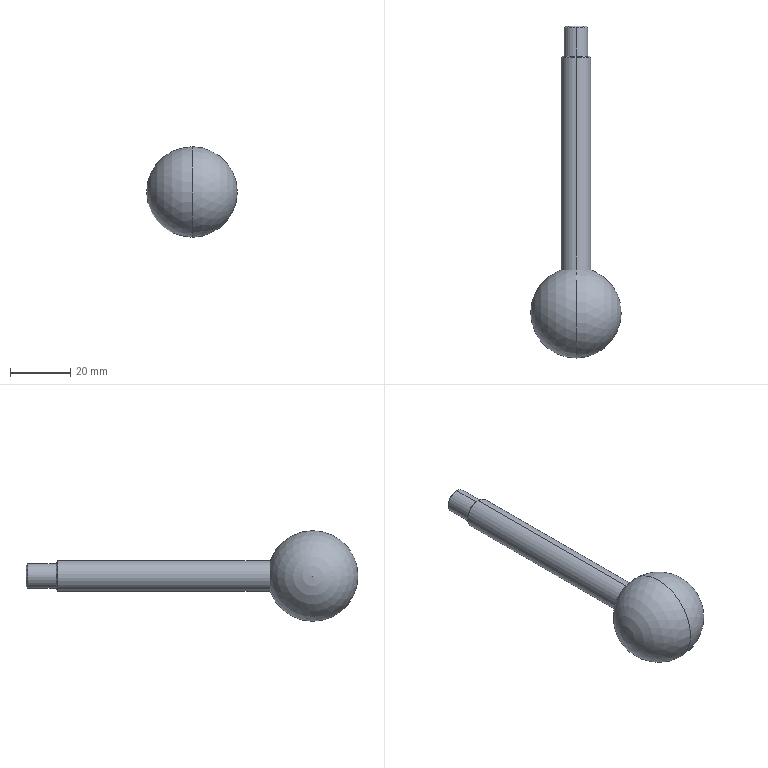Part | STEP file | M8 handle_SUS304 | 1 solid | 12 faces | box 30 x 110 x 30 mm | volume 20164 mm3 | cylinder 4 | cone 4 | sphere 2 | plane 2 | commonest cylinder face diameters 8 x2 10 x2
STEP:
#1=CARTESIAN_POINT('',(0.,0.,0.));
#2=DIRECTION('',(0.,0.,1.));
#3=DIRECTION('',(1.,0.,0.));
#4=AXIS2_PLACEMENT_3D('',#1,#2,#3);
#5=CARTESIAN_POINT('',(0.,-15.,0.));
#6=VERTEX_POINT('',#5);
#7=CARTESIAN_POINT('',(0.,0.,15.));
#8=VERTEX_POINT('',#7);
#9=CARTESIAN_POINT('',(0.,0.,0.));
#10=DIRECTION('',(-1.,0.,0.));
#11=DIRECTION('',(0.,-1.,0.));
#12=AXIS2_PLACEMENT_3D('',#9,#10,#11);
#13=CIRCLE('',#12,15.);
#14=CARTESIAN_POINT('',(0.,0.,0.));
#15=DIRECTION('',(1.,0.,0.));
#16=DIRECTION('',(0.,-1.,0.));
#17=AXIS2_PLACEMENT_3D('',#14,#15,#16);
#18=SPHERICAL_SURFACE('',#17,15.);
#19=CARTESIAN_POINT('',(6.283,0.));
#20=CARTESIAN_POINT('',(6.236,0.));
#21=CARTESIAN_POINT('',(6.14,0.));
#22=CARTESIAN_POINT('',(5.998,0.));
#23=CARTESIAN_POINT('',(5.855,0.));
#24=CARTESIAN_POINT('',(5.712,0.));
#25=CARTESIAN_POINT('',(5.569,0.));
#26=CARTESIAN_POINT('',(5.426,0.));
#27=CARTESIAN_POINT('',(5.284,0.));
#28=CARTESIAN_POINT('',(5.141,0.));
#29=CARTESIAN_POINT('',(4.998,0.));
#30=CARTESIAN_POINT('',(4.855,0.));
#31=CARTESIAN_POINT('',(4.76,0.));
#32=CARTESIAN_POINT('',(4.712,0.));
#33=B_SPLINE_CURVE_WITH_KNOTS('',3,(#19,#20,#21,#22,#23,#24,#25,#26,#27,#28,#29,#30,#31,#32),.UNSPECIFIED.,.F.,.F.,(4,1,1,1,1,1,1,1,1,1,1,4),(0.,0.1428,0.2856,0.4284,0.5712,0.714,0.8568,0.9996,1.142,1.285,1.428,1.571),.QUASI_UNIFORM_KNOTS.);
#34=(GEOMETRIC_REPRESENTATION_CONTEXT(2)PARAMETRIC_REPRESENTATION_CONTEXT()REPRESENTATION_CONTEXT('',''));
#35=DEFINITIONAL_REPRESENTATION('',(#33),#34);
#36=PCURVE('',#18,#35);
#37=CARTESIAN_POINT('',(0.,0.,0.));
#38=DIRECTION('',(1.,0.,0.));
#39=DIRECTION('',(0.,-1.,0.));
#40=AXIS2_PLACEMENT_3D('',#37,#38,#39);
#41=SPHERICAL_SURFACE('',#40,15.);
#42=CARTESIAN_POINT('',(6.283,0.));
#43=CARTESIAN_POINT('',(6.259,0.));
#44=CARTESIAN_POINT('',(6.212,0.));
#45=CARTESIAN_POINT('',(6.14,0.));
#46=CARTESIAN_POINT('',(6.069,0.));
#47=CARTESIAN_POINT('',(5.998,0.));
#48=CARTESIAN_POINT('',(5.926,0.));
#49=CARTESIAN_POINT('',(5.855,0.));
#50=CARTESIAN_POINT('',(5.783,0.));
#51=CARTESIAN_POINT('',(5.712,0.));
#52=CARTESIAN_POINT('',(5.641,0.));
#53=CARTESIAN_POINT('',(5.569,0.));
#54=CARTESIAN_POINT('',(5.498,0.));
#55=CARTESIAN_POINT('',(5.426,0.));
#56=CARTESIAN_POINT('',(5.355,0.));
#57=CARTESIAN_POINT('',(5.284,0.));
#58=CARTESIAN_POINT('',(5.212,0.));
#59=CARTESIAN_POINT('',(5.141,0.));
#60=CARTESIAN_POINT('',(5.069,0.));
#61=CARTESIAN_POINT('',(4.998,0.));
#62=CARTESIAN_POINT('',(4.927,0.));
#63=CARTESIAN_POINT('',(4.855,0.));
#64=CARTESIAN_POINT('',(4.784,0.));
#65=CARTESIAN_POINT('',(4.736,0.));
#66=CARTESIAN_POINT('',(4.712,0.));
#67=B_SPLINE_CURVE_WITH_KNOTS('',3,(#42,#43,#44,#45,#46,#47,#48,#49,#50,#51,#52,#53,#54,#55,#56,#57,#58,#59,#60,#61,#62,#63,#64,#65,#66),.UNSPECIFIED.,.F.,.F.,(4,1,1,1,1,1,1,1,1,1,1,1,1,1,1,1,1,1,1,1,1,1,4),(0.,0.0714,0.1428,0.2142,0.2856,0.357,0.4284,0.4998,0.5712,0.6426,0.714,0.7854,0.8568,0.9282,0.9996,1.071,1.142,1.214,1.285,1.357,1.428,1.499,1.571),.QUASI_UNIFORM_KNOTS.);
#68=(GEOMETRIC_REPRESENTATION_CONTEXT(2)PARAMETRIC_REPRESENTATION_CONTEXT()REPRESENTATION_CONTEXT('',''));
#69=DEFINITIONAL_REPRESENTATION('',(#67),#68);
#70=PCURVE('',#41,#69);
#71=SURFACE_CURVE('',#13,(#36,#70),.PCURVE_S1.);
#72=EDGE_CURVE('',#6,#8,#71,.T.);
#73=ORIENTED_EDGE('',*,*,#72,.F.);
#74=CARTESIAN_POINT('',(15.,0.,0.));
#75=VERTEX_POINT('',#74);
#76=CARTESIAN_POINT('',(0.,-15.,0.));
#77=CARTESIAN_POINT('',(3.366,-15.,0.));
#78=CARTESIAN_POINT('',(6.732,-14.119,0.));
#79=CARTESIAN_POINT('',(9.821,-12.356,0.));
#80=CARTESIAN_POINT('',(12.356,-9.821,0.));
#81=CARTESIAN_POINT('',(14.119,-6.732,0.));
#82=CARTESIAN_POINT('',(15.,-3.366,0.));
#83=CARTESIAN_POINT('',(15.,0.,0.));
#84=B_SPLINE_CURVE_WITH_KNOTS('',7,(#76,#77,#78,#79,#80,#81,#82,#83),.UNSPECIFIED.,.F.,.F.,(8,8),(0.,1.571),.PIECEWISE_BEZIER_KNOTS.);
#85=CARTESIAN_POINT('',(6.283,0.));
#86=DIRECTION('',(0.,1.));
#87=VECTOR('',#86,1.);
#88=LINE('',#85,#87);
#89=(GEOMETRIC_REPRESENTATION_CONTEXT(2)PARAMETRIC_REPRESENTATION_CONTEXT()REPRESENTATION_CONTEXT('',''));
#90=DEFINITIONAL_REPRESENTATION('',(#88),#89);
#91=PCURVE('',#18,#90);
#92=CARTESIAN_POINT('',(0.,0.));
#93=DIRECTION('',(0.,1.));
#94=VECTOR('',#93,1.);
#95=LINE('',#92,#94);
#96=(GEOMETRIC_REPRESENTATION_CONTEXT(2)PARAMETRIC_REPRESENTATION_CONTEXT()REPRESENTATION_CONTEXT('',''));
#97=DEFINITIONAL_REPRESENTATION('',(#95),#96);
#98=PCURVE('',#18,#97);
#99=SEAM_CURVE('',#84,(#91,#98),.PCURVE_S1.);
#100=EDGE_CURVE('',#6,#75,#99,.T.);
#101=ORIENTED_EDGE('',*,*,#100,.T.);
#102=ORIENTED_EDGE('',*,*,#100,.F.);
#103=CARTESIAN_POINT('',(0.,0.,-15.));
#104=VERTEX_POINT('',#103);
#105=CARTESIAN_POINT('',(0.,0.,0.));
#106=DIRECTION('',(-1.,0.,0.));
#107=DIRECTION('',(0.,-1.,0.));
#108=AXIS2_PLACEMENT_3D('',#105,#106,#107);
#109=CIRCLE('',#108,15.);
#110=CARTESIAN_POINT('',(1.571,0.));
#111=CARTESIAN_POINT('',(1.523,0.));
#112=CARTESIAN_POINT('',(1.428,0.));
#113=CARTESIAN_POINT('',(1.285,0.));
#114=CARTESIAN_POINT('',(1.142,0.));
#115=CARTESIAN_POINT('',(0.9996,0.));
#116=CARTESIAN_POINT('',(0.8568,0.));
#117=CARTESIAN_POINT('',(0.714,0.));
#118=CARTESIAN_POINT('',(0.5712,0.));
#119=CARTESIAN_POINT('',(0.4284,0.));
#120=CARTESIAN_POINT('',(0.2856,0.));
#121=CARTESIAN_POINT('',(0.1428,0.));
#122=CARTESIAN_POINT('',(0.,0.));
#123=CARTESIAN_POINT('',(-0.1428,0.));
#124=CARTESIAN_POINT('',(-0.2856,0.));
#125=CARTESIAN_POINT('',(-0.4284,0.));
#126=CARTESIAN_POINT('',(-0.5712,0.));
#127=CARTESIAN_POINT('',(-0.714,0.));
#128=CARTESIAN_POINT('',(-0.8568,0.));
#129=CARTESIAN_POINT('',(-0.9996,0.));
#130=CARTESIAN_POINT('',(-1.142,0.));
#131=CARTESIAN_POINT('',(-1.285,0.));
#132=CARTESIAN_POINT('',(-1.428,0.));
#133=CARTESIAN_POINT('',(-1.523,0.));
#134=CARTESIAN_POINT('',(-1.571,0.));
#135=B_SPLINE_CURVE_WITH_KNOTS('',3,(#110,#111,#112,#113,#114,#115,#116,#117,#118,#119,#120,#121,#122,#123,#124,#125,#126,#127,#128,#129,#130,#131,#132,#133,#134),.UNSPECIFIED.,.F.,.F.,(4,1,1,1,1,1,1,1,1,1,1,1,1,1,1,1,1,1,1,1,1,1,4),(4.712,4.855,4.998,5.141,5.284,5.426,5.569,5.712,5.855,5.998,6.14,6.283,6.426,6.569,6.712,6.854,6.997,7.14,7.283,7.426,7.568,7.711,7.854),.QUASI_UNIFORM_KNOTS.);
#136=(GEOMETRIC_REPRESENTATION_CONTEXT(2)PARAMETRIC_REPRESENTATION_CONTEXT()REPRESENTATION_CONTEXT('',''));
#137=DEFINITIONAL_REPRESENTATION('',(#135),#136);
#138=PCURVE('',#18,#137);
#139=CARTESIAN_POINT('',(1.571,0.));
#140=CARTESIAN_POINT('',(1.547,0.));
#141=CARTESIAN_POINT('',(1.499,0.));
#142=CARTESIAN_POINT('',(1.428,0.));
#143=CARTESIAN_POINT('',(1.357,0.));
#144=CARTESIAN_POINT('',(1.285,0.));
#145=CARTESIAN_POINT('',(1.214,0.));
#146=CARTESIAN_POINT('',(1.142,0.));
#147=CARTESIAN_POINT('',(1.071,0.));
#148=CARTESIAN_POINT('',(0.9996,0.));
#149=CARTESIAN_POINT('',(0.9282,0.));
#150=CARTESIAN_POINT('',(0.8568,0.));
#151=CARTESIAN_POINT('',(0.7854,0.));
#152=CARTESIAN_POINT('',(0.714,0.));
#153=CARTESIAN_POINT('',(0.6426,0.));
#154=CARTESIAN_POINT('',(0.5712,0.));
#155=CARTESIAN_POINT('',(0.4998,0.));
#156=CARTESIAN_POINT('',(0.4284,0.));
#157=CARTESIAN_POINT('',(0.357,0.));
#158=CARTESIAN_POINT('',(0.2856,0.));
#159=CARTESIAN_POINT('',(0.2142,0.));
#160=CARTESIAN_POINT('',(0.1428,0.));
#161=CARTESIAN_POINT('',(0.0714,0.));
#162=CARTESIAN_POINT('',(0.0238,0.));
#163=CARTESIAN_POINT('',(0.,0.));
#164=B_SPLINE_CURVE_WITH_KNOTS('',3,(#139,#140,#141,#142,#143,#144,#145,#146,#147,#148,#149,#150,#151,#152,#153,#154,#155,#156,#157,#158,#159,#160,#161,#162,#163),.UNSPECIFIED.,.F.,.F.,(4,1,1,1,1,1,1,1,1,1,1,1,1,1,1,1,1,1,1,1,1,1,4),(4.712,4.784,4.855,4.927,4.998,5.069,5.141,5.212,5.284,5.355,5.426,5.498,5.569,5.641,5.712,5.783,5.855,5.926,5.998,6.069,6.14,6.212,6.283),.QUASI_UNIFORM_KNOTS.);
#165=(GEOMETRIC_REPRESENTATION_CONTEXT(2)PARAMETRIC_REPRESENTATION_CONTEXT()REPRESENTATION_CONTEXT('',''));
#166=DEFINITIONAL_REPRESENTATION('',(#164),#165);
#167=PCURVE('',#41,#166);
#168=SURFACE_CURVE('',#109,(#138,#167),.PCURVE_S1.);
#169=EDGE_CURVE('',#104,#6,#168,.T.);
#170=ORIENTED_EDGE('',*,*,#169,.F.);
#171=CARTESIAN_POINT('',(0.,14.142,-5.));
#172=VERTEX_POINT('',#171);
#173=CARTESIAN_POINT('',(0.,0.,0.));
#174=DIRECTION('',(1.,0.,0.));
#175=DIRECTION('',(0.,1.,0.));
#176=AXIS2_PLACEMENT_3D('',#173,#174,#175);
#177=CIRCLE('',#176,15.);
#178=CARTESIAN_POINT('',(-3.142,0.));
#179=DIRECTION('',(1.,0.));
#180=VECTOR('',#179,1.);
#181=LINE('',#178,#180);
#182=(GEOMETRIC_REPRESENTATION_CONTEXT(2)PARAMETRIC_REPRESENTATION_CONTEXT()REPRESENTATION_CONTEXT('',''));
#183=DEFINITIONAL_REPRESENTATION('',(#181),#182);
#184=PCURVE('',#18,#183);
#185=CARTESIAN_POINT('',(-3.142,0.));
#186=DIRECTION('',(1.,0.));
#187=VECTOR('',#186,1.);
#188=LINE('',#185,#187);
#189=(GEOMETRIC_REPRESENTATION_CONTEXT(2)PARAMETRIC_REPRESENTATION_CONTEXT()REPRESENTATION_CONTEXT('',''));
#190=DEFINITIONAL_REPRESENTATION('',(#188),#189);
#191=PCURVE('',#41,#190);
#192=SURFACE_CURVE('',#177,(#184,#191),.PCURVE_S1.);
#193=EDGE_CURVE('',#104,#172,#192,.T.);
#194=ORIENTED_EDGE('',*,*,#193,.T.);
#195=CARTESIAN_POINT('',(0.,14.142,5.));
#196=VERTEX_POINT('',#195);
#197=CARTESIAN_POINT('',(0.,14.142,0.));
#198=DIRECTION('',(0.,-1.,0.));
#199=DIRECTION('',(0.,0.,-1.));
#200=AXIS2_PLACEMENT_3D('',#197,#198,#199);
#201=CIRCLE('',#200,5.);
#202=CARTESIAN_POINT('',(2.802,0.));
#203=CARTESIAN_POINT('',(2.802,0.01587));
#204=CARTESIAN_POINT('',(2.804,0.0476));
#205=CARTESIAN_POINT('',(2.813,0.09434));
#206=CARTESIAN_POINT('',(2.829,0.1393));
#207=CARTESIAN_POINT('',(2.852,0.1818));
#208=CARTESIAN_POINT('',(2.88,0.2208));
#209=CARTESIAN_POINT('',(2.913,0.2555));
#210=CARTESIAN_POINT('',(2.952,0.2852));
#211=CARTESIAN_POINT('',(2.995,0.3091));
#212=CARTESIAN_POINT('',(3.042,0.3267));
#213=CARTESIAN_POINT('',(3.091,0.3374));
#214=CARTESIAN_POINT('',(3.142,0.341));
#215=CARTESIAN_POINT('',(3.192,0.3374));
#216=CARTESIAN_POINT('',(3.241,0.3267));
#217=CARTESIAN_POINT('',(3.288,0.3091));
#218=CARTESIAN_POINT('',(3.331,0.2852));
#219=CARTESIAN_POINT('',(3.37,0.2555));
#220=CARTESIAN_POINT('',(3.404,0.2208));
#221=CARTESIAN_POINT('',(3.432,0.1818));
#222=CARTESIAN_POINT('',(3.454,0.1393));
#223=CARTESIAN_POINT('',(3.47,0.09434));
#224=CARTESIAN_POINT('',(3.479,0.0476));
#225=CARTESIAN_POINT('',(3.481,0.01587));
#226=CARTESIAN_POINT('',(3.481,0.));
#227=B_SPLINE_CURVE_WITH_KNOTS('',3,(#202,#203,#204,#205,#206,#207,#208,#209,#210,#211,#212,#213,#214,#215,#216,#217,#218,#219,#220,#221,#222,#223,#224,#225,#226),.UNSPECIFIED.,.F.,.F.,(4,1,1,1,1,1,1,1,1,1,1,1,1,1,1,1,1,1,1,1,1,1,4),(0.,0.1428,0.2856,0.4284,0.5712,0.714,0.8568,0.9996,1.142,1.285,1.428,1.571,1.714,1.856,1.999,2.142,2.285,2.428,2.57,2.713,2.856,2.999,3.142),.QUASI_UNIFORM_KNOTS.);
#228=(GEOMETRIC_REPRESENTATION_CONTEXT(2)PARAMETRIC_REPRESENTATION_CONTEXT()REPRESENTATION_CONTEXT('',''));
#229=DEFINITIONAL_REPRESENTATION('',(#227),#228);
#230=PCURVE('',#18,#229);
#231=CARTESIAN_POINT('',(0.,85.,0.));
#232=DIRECTION('',(0.,-1.,0.));
#233=DIRECTION('',(0.,0.,-1.));
#234=AXIS2_PLACEMENT_3D('',#231,#232,#233);
#235=CYLINDRICAL_SURFACE('',#234,5.);
#236=CARTESIAN_POINT('',(0.,70.858));
#237=DIRECTION('',(1.,0.));
#238=VECTOR('',#237,1.);
#239=LINE('',#236,#238);
#240=(GEOMETRIC_REPRESENTATION_CONTEXT(2)PARAMETRIC_REPRESENTATION_CONTEXT()REPRESENTATION_CONTEXT('',''));
#241=DEFINITIONAL_REPRESENTATION('',(#239),#240);
#242=PCURVE('',#235,#241);
#243=SURFACE_CURVE('',#201,(#230,#242),.PCURVE_S1.);
#244=EDGE_CURVE('',#172,#196,#243,.T.);
#245=ORIENTED_EDGE('',*,*,#244,.T.);
#246=CARTESIAN_POINT('',(0.,0.,0.));
#247=DIRECTION('',(1.,0.,0.));
#248=DIRECTION('',(0.,1.,0.));
#249=AXIS2_PLACEMENT_3D('',#246,#247,#248);
#250=CIRCLE('',#249,15.);
#251=CARTESIAN_POINT('',(3.142,0.));
#252=DIRECTION('',(1.,0.));
#253=VECTOR('',#252,1.);
#254=LINE('',#251,#253);
#255=(GEOMETRIC_REPRESENTATION_CONTEXT(2)PARAMETRIC_REPRESENTATION_CONTEXT()REPRESENTATION_CONTEXT('',''));
#256=DEFINITIONAL_REPRESENTATION('',(#254),#255);
#257=PCURVE('',#18,#256);
#258=CARTESIAN_POINT('',(3.142,0.));
#259=DIRECTION('',(1.,0.));
#260=VECTOR('',#259,1.);
#261=LINE('',#258,#260);
#262=(GEOMETRIC_REPRESENTATION_CONTEXT(2)PARAMETRIC_REPRESENTATION_CONTEXT()REPRESENTATION_CONTEXT('',''));
#263=DEFINITIONAL_REPRESENTATION('',(#261),#262);
#264=PCURVE('',#41,#263);
#265=SURFACE_CURVE('',#250,(#257,#264),.PCURVE_S1.);
#266=EDGE_CURVE('',#196,#8,#265,.T.);
#267=ORIENTED_EDGE('',*,*,#266,.T.);
#268=EDGE_LOOP('',(#73,#101,#102,#170,#194,#245,#267));
#269=FACE_BOUND('',#268,.T.);
#270=ADVANCED_FACE('',(#269),#18,.T.);
#271=CARTESIAN_POINT('',(0.,84.5,-5.));
#272=VERTEX_POINT('',#271);
#273=CARTESIAN_POINT('',(0.,84.5,5.));
#274=VERTEX_POINT('',#273);
#275=CARTESIAN_POINT('',(0.,84.5,0.));
#276=DIRECTION('',(0.,-1.,0.));
#277=DIRECTION('',(0.,0.,-1.));
#278=AXIS2_PLACEMENT_3D('',#275,#276,#277);
#279=CIRCLE('',#278,5.);
#280=CARTESIAN_POINT('',(0.,0.5));
#281=DIRECTION('',(1.,0.));
#282=VECTOR('',#281,1.);
#283=LINE('',#280,#282);
#284=(GEOMETRIC_REPRESENTATION_CONTEXT(2)PARAMETRIC_REPRESENTATION_CONTEXT()REPRESENTATION_CONTEXT('',''));
#285=DEFINITIONAL_REPRESENTATION('',(#283),#284);
#286=PCURVE('',#235,#285);
#287=CARTESIAN_POINT('',(0.,84.5,0.));
#288=DIRECTION('',(0.,-1.,0.));
#289=DIRECTION('',(0.,0.,-1.));
#290=AXIS2_PLACEMENT_3D('',#287,#288,#289);
#291=CONICAL_SURFACE('',#290,5.,0.7854);
#292=CARTESIAN_POINT('',(0.,0.));
#293=DIRECTION('',(1.,0.));
#294=VECTOR('',#293,1.);
#295=LINE('',#292,#294);
#296=(GEOMETRIC_REPRESENTATION_CONTEXT(2)PARAMETRIC_REPRESENTATION_CONTEXT()REPRESENTATION_CONTEXT('',''));
#297=DEFINITIONAL_REPRESENTATION('',(#295),#296);
#298=PCURVE('',#291,#297);
#299=SURFACE_CURVE('',#279,(#286,#298),.PCURVE_S1.);
#300=EDGE_CURVE('',#272,#274,#299,.T.);
#301=ORIENTED_EDGE('',*,*,#300,.T.);
#302=CARTESIAN_POINT('',(0.,85.,5.));
#303=DIRECTION('',(0.,-1.,0.));
#304=VECTOR('',#303,1.);
#305=LINE('',#302,#304);
#306=CARTESIAN_POINT('',(3.142,0.));
#307=DIRECTION('',(0.,1.));
#308=VECTOR('',#307,1.);
#309=LINE('',#306,#308);
#310=(GEOMETRIC_REPRESENTATION_CONTEXT(2)PARAMETRIC_REPRESENTATION_CONTEXT()REPRESENTATION_CONTEXT('',''));
#311=DEFINITIONAL_REPRESENTATION('',(#309),#310);
#312=PCURVE('',#235,#311);
#313=CARTESIAN_POINT('',(0.,85.,0.));
#314=DIRECTION('',(0.,-1.,0.));
#315=DIRECTION('',(0.,0.,-1.));
#316=AXIS2_PLACEMENT_3D('',#313,#314,#315);
#317=CYLINDRICAL_SURFACE('',#316,5.);
#318=CARTESIAN_POINT('',(3.142,0.));
#319=DIRECTION('',(0.,1.));
#320=VECTOR('',#319,1.);
#321=LINE('',#318,#320);
#322=(GEOMETRIC_REPRESENTATION_CONTEXT(2)PARAMETRIC_REPRESENTATION_CONTEXT()REPRESENTATION_CONTEXT('',''));
#323=DEFINITIONAL_REPRESENTATION('',(#321),#322);
#324=PCURVE('',#317,#323);
#325=SURFACE_CURVE('',#305,(#312,#324),.PCURVE_S1.);
#326=EDGE_CURVE('',#274,#196,#325,.T.);
#327=ORIENTED_EDGE('',*,*,#326,.T.);
#328=ORIENTED_EDGE('',*,*,#244,.F.);
#329=CARTESIAN_POINT('',(0.,85.,-5.));
#330=DIRECTION('',(0.,-1.,0.));
#331=VECTOR('',#330,1.);
#332=LINE('',#329,#331);
#333=CARTESIAN_POINT('',(0.,0.));
#334=DIRECTION('',(0.,1.));
#335=VECTOR('',#334,1.);
#336=LINE('',#333,#335);
#337=(GEOMETRIC_REPRESENTATION_CONTEXT(2)PARAMETRIC_REPRESENTATION_CONTEXT()REPRESENTATION_CONTEXT('',''));
#338=DEFINITIONAL_REPRESENTATION('',(#336),#337);
#339=PCURVE('',#235,#338);
#340=CARTESIAN_POINT('',(6.283,0.));
#341=DIRECTION('',(0.,1.));
#342=VECTOR('',#341,1.);
#343=LINE('',#340,#342);
#344=(GEOMETRIC_REPRESENTATION_CONTEXT(2)PARAMETRIC_REPRESENTATION_CONTEXT()REPRESENTATION_CONTEXT('',''));
#345=DEFINITIONAL_REPRESENTATION('',(#343),#344);
#346=PCURVE('',#317,#345);
#347=SURFACE_CURVE('',#332,(#339,#346),.PCURVE_S1.);
#348=EDGE_CURVE('',#272,#172,#347,.T.);
#349=ORIENTED_EDGE('',*,*,#348,.F.);
#350=EDGE_LOOP('',(#301,#327,#328,#349));
#351=FACE_BOUND('',#350,.T.);
#352=ADVANCED_FACE('',(#351),#235,.T.);
#353=CARTESIAN_POINT('',(0.,85.,-4.5));
#354=VERTEX_POINT('',#353);
#355=CARTESIAN_POINT('',(0.,85.,4.5));
#356=VERTEX_POINT('',#355);
#357=CARTESIAN_POINT('',(0.,85.,0.));
#358=DIRECTION('',(0.,-1.,0.));
#359=DIRECTION('',(0.,0.,-1.));
#360=AXIS2_PLACEMENT_3D('',#357,#358,#359);
#361=CIRCLE('',#360,4.5);
#362=CARTESIAN_POINT('',(0.,-0.5));
#363=DIRECTION('',(1.,0.));
#364=VECTOR('',#363,1.);
#365=LINE('',#362,#364);
#366=(GEOMETRIC_REPRESENTATION_CONTEXT(2)PARAMETRIC_REPRESENTATION_CONTEXT()REPRESENTATION_CONTEXT('',''));
#367=DEFINITIONAL_REPRESENTATION('',(#365),#366);
#368=PCURVE('',#291,#367);
#369=CARTESIAN_POINT('',(0.,85.,0.));
#370=DIRECTION('',(0.,1.,0.));
#371=DIRECTION('',(0.,0.,1.));
#372=AXIS2_PLACEMENT_3D('',#369,#370,#371);
#373=PLANE('',#372);
#374=CARTESIAN_POINT('',(-4.5,0.));
#375=CARTESIAN_POINT('',(-4.5,7.794));
#376=CARTESIAN_POINT('',(2.25,3.897));
#377=CARTESIAN_POINT('',(9.,0.));
#378=CARTESIAN_POINT('',(2.25,-3.897));
#379=CARTESIAN_POINT('',(-4.5,-7.794));
#380=CARTESIAN_POINT('',(-4.5,0.));
#381=(BOUNDED_CURVE()B_SPLINE_CURVE(2,(#374,#375,#376,#377,#378,#379,#380),.UNSPECIFIED.,.T.,.F.)B_SPLINE_CURVE_WITH_KNOTS((1,2,2,2,2,1),(-2.094,0.,2.094,4.189,6.283,8.378),.UNSPECIFIED.)CURVE()GEOMETRIC_REPRESENTATION_ITEM()RATIONAL_B_SPLINE_CURVE((1.,0.5,1.,0.5,1.,0.5,1.))REPRESENTATION_ITEM(''));
#382=(GEOMETRIC_REPRESENTATION_CONTEXT(2)PARAMETRIC_REPRESENTATION_CONTEXT()REPRESENTATION_CONTEXT('',''));
#383=DEFINITIONAL_REPRESENTATION('',(#381),#382);
#384=PCURVE('',#373,#383);
#385=SURFACE_CURVE('',#361,(#368,#384),.PCURVE_S1.);
#386=EDGE_CURVE('',#354,#356,#385,.T.);
#387=ORIENTED_EDGE('',*,*,#386,.T.);
#388=CARTESIAN_POINT('',(0.,84.5,5.));
#389=DIRECTION('',(0.,-0.7071,0.7071));
#390=VECTOR('',#389,1.);
#391=LINE('',#388,#390);
#392=CARTESIAN_POINT('',(3.142,0.));
#393=DIRECTION('',(0.,1.));
#394=VECTOR('',#393,1.);
#395=LINE('',#392,#394);
#396=(GEOMETRIC_REPRESENTATION_CONTEXT(2)PARAMETRIC_REPRESENTATION_CONTEXT()REPRESENTATION_CONTEXT('',''));
#397=DEFINITIONAL_REPRESENTATION('',(#395),#396);
#398=PCURVE('',#291,#397);
#399=CARTESIAN_POINT('',(0.,84.5,0.));
#400=DIRECTION('',(0.,-1.,0.));
#401=DIRECTION('',(0.,0.,-1.));
#402=AXIS2_PLACEMENT_3D('',#399,#400,#401);
#403=CONICAL_SURFACE('',#402,5.,0.7854);
#404=CARTESIAN_POINT('',(3.142,0.));
#405=DIRECTION('',(0.,1.));
#406=VECTOR('',#405,1.);
#407=LINE('',#404,#406);
#408=(GEOMETRIC_REPRESENTATION_CONTEXT(2)PARAMETRIC_REPRESENTATION_CONTEXT()REPRESENTATION_CONTEXT('',''));
#409=DEFINITIONAL_REPRESENTATION('',(#407),#408);
#410=PCURVE('',#403,#409);
#411=SURFACE_CURVE('',#391,(#398,#410),.PCURVE_S1.);
#412=EDGE_CURVE('',#356,#274,#411,.T.);
#413=ORIENTED_EDGE('',*,*,#412,.T.);
#414=ORIENTED_EDGE('',*,*,#300,.F.);
#415=CARTESIAN_POINT('',(0.,84.5,-5.));
#416=DIRECTION('',(0.,-0.7071,-0.7071));
#417=VECTOR('',#416,1.);
#418=LINE('',#415,#417);
#419=CARTESIAN_POINT('',(0.,0.));
#420=DIRECTION('',(0.,1.));
#421=VECTOR('',#420,1.);
#422=LINE('',#419,#421);
#423=(GEOMETRIC_REPRESENTATION_CONTEXT(2)PARAMETRIC_REPRESENTATION_CONTEXT()REPRESENTATION_CONTEXT('',''));
#424=DEFINITIONAL_REPRESENTATION('',(#422),#423);
#425=PCURVE('',#291,#424);
#426=CARTESIAN_POINT('',(6.283,0.));
#427=DIRECTION('',(0.,1.));
#428=VECTOR('',#427,1.);
#429=LINE('',#426,#428);
#430=(GEOMETRIC_REPRESENTATION_CONTEXT(2)PARAMETRIC_REPRESENTATION_CONTEXT()REPRESENTATION_CONTEXT('',''));
#431=DEFINITIONAL_REPRESENTATION('',(#429),#430);
#432=PCURVE('',#403,#431);
#433=SURFACE_CURVE('',#418,(#425,#432),.PCURVE_S1.);
#434=EDGE_CURVE('',#354,#272,#433,.T.);
#435=ORIENTED_EDGE('',*,*,#434,.F.);
#436=EDGE_LOOP('',(#387,#413,#414,#435));
#437=FACE_BOUND('',#436,.T.);
#438=ADVANCED_FACE('',(#437),#291,.T.);
#439=CARTESIAN_POINT('',(0.,94.5,-4.));
#440=VERTEX_POINT('',#439);
#441=CARTESIAN_POINT('',(0.,94.5,4.));
#442=VERTEX_POINT('',#441);
#443=CARTESIAN_POINT('',(0.,94.5,0.));
#444=DIRECTION('',(0.,-1.,0.));
#445=DIRECTION('',(0.,0.,-1.));
#446=AXIS2_PLACEMENT_3D('',#443,#444,#445);
#447=CIRCLE('',#446,4.);
#448=CARTESIAN_POINT('',(0.,95.,0.));
#449=DIRECTION('',(0.,-1.,0.));
#450=DIRECTION('',(0.,0.,-1.));
#451=AXIS2_PLACEMENT_3D('',#448,#449,#450);
#452=CYLINDRICAL_SURFACE('',#451,4.);
#453=CARTESIAN_POINT('',(0.,0.5));
#454=DIRECTION('',(1.,0.));
#455=VECTOR('',#454,1.);
#456=LINE('',#453,#455);
#457=(GEOMETRIC_REPRESENTATION_CONTEXT(2)PARAMETRIC_REPRESENTATION_CONTEXT()REPRESENTATION_CONTEXT('',''));
#458=DEFINITIONAL_REPRESENTATION('',(#456),#457);
#459=PCURVE('',#452,#458);
#460=CARTESIAN_POINT('',(0.,94.5,0.));
#461=DIRECTION('',(0.,-1.,0.));
#462=DIRECTION('',(0.,0.,-1.));
#463=AXIS2_PLACEMENT_3D('',#460,#461,#462);
#464=CONICAL_SURFACE('',#463,4.,0.7854);
#465=CARTESIAN_POINT('',(0.,0.));
#466=DIRECTION('',(1.,0.));
#467=VECTOR('',#466,1.);
#468=LINE('',#465,#467);
#469=(GEOMETRIC_REPRESENTATION_CONTEXT(2)PARAMETRIC_REPRESENTATION_CONTEXT()REPRESENTATION_CONTEXT('',''));
#470=DEFINITIONAL_REPRESENTATION('',(#468),#469);
#471=PCURVE('',#464,#470);
#472=SURFACE_CURVE('',#447,(#459,#471),.PCURVE_S1.);
#473=EDGE_CURVE('',#440,#442,#472,.T.);
#474=ORIENTED_EDGE('',*,*,#473,.T.);
#475=CARTESIAN_POINT('',(0.,85.,4.));
#476=VERTEX_POINT('',#475);
#477=CARTESIAN_POINT('',(0.,95.,4.));
#478=DIRECTION('',(0.,-1.,0.));
#479=VECTOR('',#478,1.);
#480=LINE('',#477,#479);
#481=CARTESIAN_POINT('',(3.142,0.));
#482=DIRECTION('',(0.,1.));
#483=VECTOR('',#482,1.);
#484=LINE('',#481,#483);
#485=(GEOMETRIC_REPRESENTATION_CONTEXT(2)PARAMETRIC_REPRESENTATION_CONTEXT()REPRESENTATION_CONTEXT('',''));
#486=DEFINITIONAL_REPRESENTATION('',(#484),#485);
#487=PCURVE('',#452,#486);
#488=CARTESIAN_POINT('',(0.,95.,0.));
#489=DIRECTION('',(0.,-1.,0.));
#490=DIRECTION('',(0.,0.,-1.));
#491=AXIS2_PLACEMENT_3D('',#488,#489,#490);
#492=CYLINDRICAL_SURFACE('',#491,4.);
#493=CARTESIAN_POINT('',(3.142,0.));
#494=DIRECTION('',(0.,1.));
#495=VECTOR('',#494,1.);
#496=LINE('',#493,#495);
#497=(GEOMETRIC_REPRESENTATION_CONTEXT(2)PARAMETRIC_REPRESENTATION_CONTEXT()REPRESENTATION_CONTEXT('',''));
#498=DEFINITIONAL_REPRESENTATION('',(#496),#497);
#499=PCURVE('',#492,#498);
#500=SURFACE_CURVE('',#480,(#487,#499),.PCURVE_S1.);
#501=EDGE_CURVE('',#442,#476,#500,.T.);
#502=ORIENTED_EDGE('',*,*,#501,.T.);
#503=CARTESIAN_POINT('',(0.,85.,-4.));
#504=VERTEX_POINT('',#503);
#505=CARTESIAN_POINT('',(0.,85.,0.));
#506=DIRECTION('',(0.,-1.,0.));
#507=DIRECTION('',(0.,0.,-1.));
#508=AXIS2_PLACEMENT_3D('',#505,#506,#507);
#509=CIRCLE('',#508,4.);
#510=CARTESIAN_POINT('',(0.,10.));
#511=DIRECTION('',(1.,0.));
#512=VECTOR('',#511,1.);
#513=LINE('',#510,#512);
#514=(GEOMETRIC_REPRESENTATION_CONTEXT(2)PARAMETRIC_REPRESENTATION_CONTEXT()REPRESENTATION_CONTEXT('',''));
#515=DEFINITIONAL_REPRESENTATION('',(#513),#514);
#516=PCURVE('',#452,#515);
#517=CARTESIAN_POINT('',(-4.,0.));
#518=CARTESIAN_POINT('',(-4.,6.928));
#519=CARTESIAN_POINT('',(2.,3.464));
#520=CARTESIAN_POINT('',(8.,0.));
#521=CARTESIAN_POINT('',(2.,-3.464));
#522=CARTESIAN_POINT('',(-4.,-6.928));
#523=CARTESIAN_POINT('',(-4.,0.));
#524=(BOUNDED_CURVE()B_SPLINE_CURVE(2,(#517,#518,#519,#520,#521,#522,#523),.UNSPECIFIED.,.T.,.F.)B_SPLINE_CURVE_WITH_KNOTS((1,2,2,2,2,1),(-2.094,0.,2.094,4.189,6.283,8.378),.UNSPECIFIED.)CURVE()GEOMETRIC_REPRESENTATION_ITEM()RATIONAL_B_SPLINE_CURVE((1.,0.5,1.,0.5,1.,0.5,1.))REPRESENTATION_ITEM(''));
#525=(GEOMETRIC_REPRESENTATION_CONTEXT(2)PARAMETRIC_REPRESENTATION_CONTEXT()REPRESENTATION_CONTEXT('',''));
#526=DEFINITIONAL_REPRESENTATION('',(#524),#525);
#527=PCURVE('',#373,#526);
#528=SURFACE_CURVE('',#509,(#516,#527),.PCURVE_S1.);
#529=EDGE_CURVE('',#504,#476,#528,.T.);
#530=ORIENTED_EDGE('',*,*,#529,.F.);
#531=CARTESIAN_POINT('',(0.,95.,-4.));
#532=DIRECTION('',(0.,-1.,0.));
#533=VECTOR('',#532,1.);
#534=LINE('',#531,#533);
#535=CARTESIAN_POINT('',(0.,0.));
#536=DIRECTION('',(0.,1.));
#537=VECTOR('',#536,1.);
#538=LINE('',#535,#537);
#539=(GEOMETRIC_REPRESENTATION_CONTEXT(2)PARAMETRIC_REPRESENTATION_CONTEXT()REPRESENTATION_CONTEXT('',''));
#540=DEFINITIONAL_REPRESENTATION('',(#538),#539);
#541=PCURVE('',#452,#540);
#542=CARTESIAN_POINT('',(6.283,0.));
#543=DIRECTION('',(0.,1.));
#544=VECTOR('',#543,1.);
#545=LINE('',#542,#544);
#546=(GEOMETRIC_REPRESENTATION_CONTEXT(2)PARAMETRIC_REPRESENTATION_CONTEXT()REPRESENTATION_CONTEXT('',''));
#547=DEFINITIONAL_REPRESENTATION('',(#545),#546);
#548=PCURVE('',#492,#547);
#549=SURFACE_CURVE('',#534,(#541,#548),.PCURVE_S1.);
#550=EDGE_CURVE('',#440,#504,#549,.T.);
#551=ORIENTED_EDGE('',*,*,#550,.F.);
#552=EDGE_LOOP('',(#474,#502,#530,#551));
#553=FACE_BOUND('',#552,.T.);
#554=ADVANCED_FACE('',(#553),#452,.T.);
#555=CARTESIAN_POINT('',(0.,95.,-3.5));
#556=VERTEX_POINT('',#555);
#557=CARTESIAN_POINT('',(0.,95.,3.5));
#558=VERTEX_POINT('',#557);
#559=CARTESIAN_POINT('',(0.,95.,0.));
#560=DIRECTION('',(0.,-1.,0.));
#561=DIRECTION('',(0.,0.,-1.));
#562=AXIS2_PLACEMENT_3D('',#559,#560,#561);
#563=CIRCLE('',#562,3.5);
#564=CARTESIAN_POINT('',(0.,-0.5));
#565=DIRECTION('',(1.,0.));
#566=VECTOR('',#565,1.);
#567=LINE('',#564,#566);
#568=(GEOMETRIC_REPRESENTATION_CONTEXT(2)PARAMETRIC_REPRESENTATION_CONTEXT()REPRESENTATION_CONTEXT('',''));
#569=DEFINITIONAL_REPRESENTATION('',(#567),#568);
#570=PCURVE('',#464,#569);
#571=CARTESIAN_POINT('',(0.,95.,0.));
#572=DIRECTION('',(0.,1.,0.));
#573=DIRECTION('',(0.,0.,1.));
#574=AXIS2_PLACEMENT_3D('',#571,#572,#573);
#575=PLANE('',#574);
#576=CARTESIAN_POINT('',(-3.5,0.));
#577=CARTESIAN_POINT('',(-3.5,6.062));
#578=CARTESIAN_POINT('',(1.75,3.031));
#579=CARTESIAN_POINT('',(7.,0.));
#580=CARTESIAN_POINT('',(1.75,-3.031));
#581=CARTESIAN_POINT('',(-3.5,-6.062));
#582=CARTESIAN_POINT('',(-3.5,0.));
#583=(BOUNDED_CURVE()B_SPLINE_CURVE(2,(#576,#577,#578,#579,#580,#581,#582),.UNSPECIFIED.,.T.,.F.)B_SPLINE_CURVE_WITH_KNOTS((1,2,2,2,2,1),(-2.094,0.,2.094,4.189,6.283,8.378),.UNSPECIFIED.)CURVE()GEOMETRIC_REPRESENTATION_ITEM()RATIONAL_B_SPLINE_CURVE((1.,0.5,1.,0.5,1.,0.5,1.))REPRESENTATION_ITEM(''));
#584=(GEOMETRIC_REPRESENTATION_CONTEXT(2)PARAMETRIC_REPRESENTATION_CONTEXT()REPRESENTATION_CONTEXT('',''));
#585=DEFINITIONAL_REPRESENTATION('',(#583),#584);
#586=PCURVE('',#575,#585);
#587=SURFACE_CURVE('',#563,(#570,#586),.PCURVE_S1.);
#588=EDGE_CURVE('',#556,#558,#587,.T.);
#589=ORIENTED_EDGE('',*,*,#588,.T.);
#590=CARTESIAN_POINT('',(0.,94.5,4.));
#591=DIRECTION('',(0.,-0.7071,0.7071));
#592=VECTOR('',#591,1.);
#593=LINE('',#590,#592);
#594=CARTESIAN_POINT('',(3.142,0.));
#595=DIRECTION('',(0.,1.));
#596=VECTOR('',#595,1.);
#597=LINE('',#594,#596);
#598=(GEOMETRIC_REPRESENTATION_CONTEXT(2)PARAMETRIC_REPRESENTATION_CONTEXT()REPRESENTATION_CONTEXT('',''));
#599=DEFINITIONAL_REPRESENTATION('',(#597),#598);
#600=PCURVE('',#464,#599);
#601=CARTESIAN_POINT('',(0.,94.5,0.));
#602=DIRECTION('',(0.,-1.,0.));
#603=DIRECTION('',(0.,0.,-1.));
#604=AXIS2_PLACEMENT_3D('',#601,#602,#603);
#605=CONICAL_SURFACE('',#604,4.,0.7854);
#606=CARTESIAN_POINT('',(3.142,0.));
#607=DIRECTION('',(0.,1.));
#608=VECTOR('',#607,1.);
#609=LINE('',#606,#608);
#610=(GEOMETRIC_REPRESENTATION_CONTEXT(2)PARAMETRIC_REPRESENTATION_CONTEXT()REPRESENTATION_CONTEXT('',''));
#611=DEFINITIONAL_REPRESENTATION('',(#609),#610);
#612=PCURVE('',#605,#611);
#613=SURFACE_CURVE('',#593,(#600,#612),.PCURVE_S1.);
#614=EDGE_CURVE('',#558,#442,#613,.T.);
#615=ORIENTED_EDGE('',*,*,#614,.T.);
#616=ORIENTED_EDGE('',*,*,#473,.F.);
#617=CARTESIAN_POINT('',(0.,94.5,-4.));
#618=DIRECTION('',(0.,-0.7071,-0.7071));
#619=VECTOR('',#618,1.);
#620=LINE('',#617,#619);
#621=CARTESIAN_POINT('',(0.,0.));
#622=DIRECTION('',(0.,1.));
#623=VECTOR('',#622,1.);
#624=LINE('',#621,#623);
#625=(GEOMETRIC_REPRESENTATION_CONTEXT(2)PARAMETRIC_REPRESENTATION_CONTEXT()REPRESENTATION_CONTEXT('',''));
#626=DEFINITIONAL_REPRESENTATION('',(#624),#625);
#627=PCURVE('',#464,#626);
#628=CARTESIAN_POINT('',(6.283,0.));
#629=DIRECTION('',(0.,1.));
#630=VECTOR('',#629,1.);
#631=LINE('',#628,#630);
#632=(GEOMETRIC_REPRESENTATION_CONTEXT(2)PARAMETRIC_REPRESENTATION_CONTEXT()REPRESENTATION_CONTEXT('',''));
#633=DEFINITIONAL_REPRESENTATION('',(#631),#632);
#634=PCURVE('',#605,#633);
#635=SURFACE_CURVE('',#620,(#627,#634),.PCURVE_S1.);
#636=EDGE_CURVE('',#556,#440,#635,.T.);
#637=ORIENTED_EDGE('',*,*,#636,.F.);
#638=EDGE_LOOP('',(#589,#615,#616,#637));
#639=FACE_BOUND('',#638,.T.);
#640=ADVANCED_FACE('',(#639),#464,.T.);
#641=ORIENTED_EDGE('',*,*,#193,.F.);
#642=ORIENTED_EDGE('',*,*,#169,.T.);
#643=CARTESIAN_POINT('',(-15.,0.,0.));
#644=VERTEX_POINT('',#643);
#645=CARTESIAN_POINT('',(-15.,0.,0.));
#646=CARTESIAN_POINT('',(-15.,-3.366,0.));
#647=CARTESIAN_POINT('',(-14.119,-6.732,0.));
#648=CARTESIAN_POINT('',(-12.356,-9.821,0.));
#649=CARTESIAN_POINT('',(-9.821,-12.356,0.));
#650=CARTESIAN_POINT('',(-6.732,-14.119,0.));
#651=CARTESIAN_POINT('',(-3.366,-15.,0.));
#652=CARTESIAN_POINT('',(0.,-15.,0.));
#653=B_SPLINE_CURVE_WITH_KNOTS('',7,(#645,#646,#647,#648,#649,#650,#651,#652),.UNSPECIFIED.,.F.,.F.,(8,8),(-1.571,0.),.PIECEWISE_BEZIER_KNOTS.);
#654=CARTESIAN_POINT('',(0.,0.));
#655=DIRECTION('',(0.,1.));
#656=VECTOR('',#655,1.);
#657=LINE('',#654,#656);
#658=(GEOMETRIC_REPRESENTATION_CONTEXT(2)PARAMETRIC_REPRESENTATION_CONTEXT()REPRESENTATION_CONTEXT('',''));
#659=DEFINITIONAL_REPRESENTATION('',(#657),#658);
#660=PCURVE('',#41,#659);
#661=CARTESIAN_POINT('',(6.283,0.));
#662=DIRECTION('',(0.,1.));
#663=VECTOR('',#662,1.);
#664=LINE('',#661,#663);
#665=(GEOMETRIC_REPRESENTATION_CONTEXT(2)PARAMETRIC_REPRESENTATION_CONTEXT()REPRESENTATION_CONTEXT('',''));
#666=DEFINITIONAL_REPRESENTATION('',(#664),#665);
#667=PCURVE('',#41,#666);
#668=SEAM_CURVE('',#653,(#660,#667),.PCURVE_S1.);
#669=EDGE_CURVE('',#644,#6,#668,.T.);
#670=ORIENTED_EDGE('',*,*,#669,.F.);
#671=ORIENTED_EDGE('',*,*,#669,.T.);
#672=ORIENTED_EDGE('',*,*,#72,.T.);
#673=ORIENTED_EDGE('',*,*,#266,.F.);
#674=CARTESIAN_POINT('',(0.,14.142,0.));
#675=DIRECTION('',(0.,-1.,0.));
#676=DIRECTION('',(0.,0.,-1.));
#677=AXIS2_PLACEMENT_3D('',#674,#675,#676);
#678=CIRCLE('',#677,5.);
#679=CARTESIAN_POINT('',(3.481,0.));
#680=CARTESIAN_POINT('',(3.481,-0.01587));
#681=CARTESIAN_POINT('',(3.479,-0.0476));
#682=CARTESIAN_POINT('',(3.47,-0.09434));
#683=CARTESIAN_POINT('',(3.454,-0.1393));
#684=CARTESIAN_POINT('',(3.432,-0.1818));
#685=CARTESIAN_POINT('',(3.404,-0.2208));
#686=CARTESIAN_POINT('',(3.37,-0.2555));
#687=CARTESIAN_POINT('',(3.331,-0.2852));
#688=CARTESIAN_POINT('',(3.288,-0.3091));
#689=CARTESIAN_POINT('',(3.241,-0.3267));
#690=CARTESIAN_POINT('',(3.192,-0.3374));
#691=CARTESIAN_POINT('',(3.142,-0.341));
#692=CARTESIAN_POINT('',(3.091,-0.3374));
#693=CARTESIAN_POINT('',(3.042,-0.3267));
#694=CARTESIAN_POINT('',(2.995,-0.3091));
#695=CARTESIAN_POINT('',(2.952,-0.2852));
#696=CARTESIAN_POINT('',(2.913,-0.2555));
#697=CARTESIAN_POINT('',(2.88,-0.2208));
#698=CARTESIAN_POINT('',(2.852,-0.1818));
#699=CARTESIAN_POINT('',(2.829,-0.1393));
#700=CARTESIAN_POINT('',(2.813,-0.09434));
#701=CARTESIAN_POINT('',(2.804,-0.0476));
#702=CARTESIAN_POINT('',(2.802,-0.01587));
#703=CARTESIAN_POINT('',(2.802,0.));
#704=B_SPLINE_CURVE_WITH_KNOTS('',3,(#679,#680,#681,#682,#683,#684,#685,#686,#687,#688,#689,#690,#691,#692,#693,#694,#695,#696,#697,#698,#699,#700,#701,#702,#703),.UNSPECIFIED.,.F.,.F.,(4,1,1,1,1,1,1,1,1,1,1,1,1,1,1,1,1,1,1,1,1,1,4),(3.142,3.284,3.427,3.57,3.713,3.856,3.998,4.141,4.284,4.427,4.57,4.712,4.855,4.998,5.141,5.284,5.426,5.569,5.712,5.855,5.998,6.14,6.283),.QUASI_UNIFORM_KNOTS.);
#705=(GEOMETRIC_REPRESENTATION_CONTEXT(2)PARAMETRIC_REPRESENTATION_CONTEXT()REPRESENTATION_CONTEXT('',''));
#706=DEFINITIONAL_REPRESENTATION('',(#704),#705);
#707=PCURVE('',#41,#706);
#708=CARTESIAN_POINT('',(0.,70.858));
#709=DIRECTION('',(1.,0.));
#710=VECTOR('',#709,1.);
#711=LINE('',#708,#710);
#712=(GEOMETRIC_REPRESENTATION_CONTEXT(2)PARAMETRIC_REPRESENTATION_CONTEXT()REPRESENTATION_CONTEXT('',''));
#713=DEFINITIONAL_REPRESENTATION('',(#711),#712);
#714=PCURVE('',#317,#713);
#715=SURFACE_CURVE('',#678,(#707,#714),.PCURVE_S1.);
#716=EDGE_CURVE('',#196,#172,#715,.T.);
#717=ORIENTED_EDGE('',*,*,#716,.T.);
#718=EDGE_LOOP('',(#641,#642,#670,#671,#672,#673,#717));
#719=FACE_BOUND('',#718,.T.);
#720=ADVANCED_FACE('',(#719),#41,.T.);
#721=ORIENTED_EDGE('',*,*,#326,.F.);
#722=CARTESIAN_POINT('',(0.,84.5,0.));
#723=DIRECTION('',(0.,-1.,0.));
#724=DIRECTION('',(0.,0.,-1.));
#725=AXIS2_PLACEMENT_3D('',#722,#723,#724);
#726=CIRCLE('',#725,5.);
#727=CARTESIAN_POINT('',(0.,0.5));
#728=DIRECTION('',(1.,0.));
#729=VECTOR('',#728,1.);
#730=LINE('',#727,#729);
#731=(GEOMETRIC_REPRESENTATION_CONTEXT(2)PARAMETRIC_REPRESENTATION_CONTEXT()REPRESENTATION_CONTEXT('',''));
#732=DEFINITIONAL_REPRESENTATION('',(#730),#731);
#733=PCURVE('',#317,#732);
#734=CARTESIAN_POINT('',(0.,0.));
#735=DIRECTION('',(1.,0.));
#736=VECTOR('',#735,1.);
#737=LINE('',#734,#736);
#738=(GEOMETRIC_REPRESENTATION_CONTEXT(2)PARAMETRIC_REPRESENTATION_CONTEXT()REPRESENTATION_CONTEXT('',''));
#739=DEFINITIONAL_REPRESENTATION('',(#737),#738);
#740=PCURVE('',#403,#739);
#741=SURFACE_CURVE('',#726,(#733,#740),.PCURVE_S1.);
#742=EDGE_CURVE('',#274,#272,#741,.T.);
#743=ORIENTED_EDGE('',*,*,#742,.T.);
#744=ORIENTED_EDGE('',*,*,#348,.T.);
#745=ORIENTED_EDGE('',*,*,#716,.F.);
#746=EDGE_LOOP('',(#721,#743,#744,#745));
#747=FACE_BOUND('',#746,.T.);
#748=ADVANCED_FACE('',(#747),#317,.T.);
#749=ORIENTED_EDGE('',*,*,#412,.F.);
#750=CARTESIAN_POINT('',(0.,85.,0.));
#751=DIRECTION('',(0.,-1.,0.));
#752=DIRECTION('',(0.,0.,-1.));
#753=AXIS2_PLACEMENT_3D('',#750,#751,#752);
#754=CIRCLE('',#753,4.5);
#755=CARTESIAN_POINT('',(0.,-0.5));
#756=DIRECTION('',(1.,0.));
#757=VECTOR('',#756,1.);
#758=LINE('',#755,#757);
#759=(GEOMETRIC_REPRESENTATION_CONTEXT(2)PARAMETRIC_REPRESENTATION_CONTEXT()REPRESENTATION_CONTEXT('',''));
#760=DEFINITIONAL_REPRESENTATION('',(#758),#759);
#761=PCURVE('',#403,#760);
#762=CARTESIAN_POINT('',(-4.5,0.));
#763=CARTESIAN_POINT('',(-4.5,7.794));
#764=CARTESIAN_POINT('',(2.25,3.897));
#765=CARTESIAN_POINT('',(9.,0.));
#766=CARTESIAN_POINT('',(2.25,-3.897));
#767=CARTESIAN_POINT('',(-4.5,-7.794));
#768=CARTESIAN_POINT('',(-4.5,0.));
#769=(BOUNDED_CURVE()B_SPLINE_CURVE(2,(#762,#763,#764,#765,#766,#767,#768),.UNSPECIFIED.,.T.,.F.)B_SPLINE_CURVE_WITH_KNOTS((1,2,2,2,2,1),(-2.094,0.,2.094,4.189,6.283,8.378),.UNSPECIFIED.)CURVE()GEOMETRIC_REPRESENTATION_ITEM()RATIONAL_B_SPLINE_CURVE((1.,0.5,1.,0.5,1.,0.5,1.))REPRESENTATION_ITEM(''));
#770=(GEOMETRIC_REPRESENTATION_CONTEXT(2)PARAMETRIC_REPRESENTATION_CONTEXT()REPRESENTATION_CONTEXT('',''));
#771=DEFINITIONAL_REPRESENTATION('',(#769),#770);
#772=PCURVE('',#373,#771);
#773=SURFACE_CURVE('',#754,(#761,#772),.PCURVE_S1.);
#774=EDGE_CURVE('',#356,#354,#773,.T.);
#775=ORIENTED_EDGE('',*,*,#774,.T.);
#776=ORIENTED_EDGE('',*,*,#434,.T.);
#777=ORIENTED_EDGE('',*,*,#742,.F.);
#778=EDGE_LOOP('',(#749,#775,#776,#777));
#779=FACE_BOUND('',#778,.T.);
#780=ADVANCED_FACE('',(#779),#403,.T.);
#781=ORIENTED_EDGE('',*,*,#386,.F.);
#782=ORIENTED_EDGE('',*,*,#774,.F.);
#783=EDGE_LOOP('',(#781,#782));
#784=FACE_BOUND('',#783,.T.);
#785=ORIENTED_EDGE('',*,*,#529,.T.);
#786=CARTESIAN_POINT('',(0.,85.,0.));
#787=DIRECTION('',(0.,-1.,0.));
#788=DIRECTION('',(0.,0.,-1.));
#789=AXIS2_PLACEMENT_3D('',#786,#787,#788);
#790=CIRCLE('',#789,4.);
#791=CARTESIAN_POINT('',(-4.,0.));
#792=CARTESIAN_POINT('',(-4.,6.928));
#793=CARTESIAN_POINT('',(2.,3.464));
#794=CARTESIAN_POINT('',(8.,0.));
#795=CARTESIAN_POINT('',(2.,-3.464));
#796=CARTESIAN_POINT('',(-4.,-6.928));
#797=CARTESIAN_POINT('',(-4.,0.));
#798=(BOUNDED_CURVE()B_SPLINE_CURVE(2,(#791,#792,#793,#794,#795,#796,#797),.UNSPECIFIED.,.T.,.F.)B_SPLINE_CURVE_WITH_KNOTS((1,2,2,2,2,1),(-2.094,0.,2.094,4.189,6.283,8.378),.UNSPECIFIED.)CURVE()GEOMETRIC_REPRESENTATION_ITEM()RATIONAL_B_SPLINE_CURVE((1.,0.5,1.,0.5,1.,0.5,1.))REPRESENTATION_ITEM(''));
#799=(GEOMETRIC_REPRESENTATION_CONTEXT(2)PARAMETRIC_REPRESENTATION_CONTEXT()REPRESENTATION_CONTEXT('',''));
#800=DEFINITIONAL_REPRESENTATION('',(#798),#799);
#801=PCURVE('',#373,#800);
#802=CARTESIAN_POINT('',(0.,10.));
#803=DIRECTION('',(1.,0.));
#804=VECTOR('',#803,1.);
#805=LINE('',#802,#804);
#806=(GEOMETRIC_REPRESENTATION_CONTEXT(2)PARAMETRIC_REPRESENTATION_CONTEXT()REPRESENTATION_CONTEXT('',''));
#807=DEFINITIONAL_REPRESENTATION('',(#805),#806);
#808=PCURVE('',#492,#807);
#809=SURFACE_CURVE('',#790,(#801,#808),.PCURVE_S1.);
#810=EDGE_CURVE('',#476,#504,#809,.T.);
#811=ORIENTED_EDGE('',*,*,#810,.T.);
#812=EDGE_LOOP('',(#785,#811));
#813=FACE_BOUND('',#812,.T.);
#814=ADVANCED_FACE('',(#784,#813),#373,.T.);
#815=ORIENTED_EDGE('',*,*,#501,.F.);
#816=CARTESIAN_POINT('',(0.,94.5,0.));
#817=DIRECTION('',(0.,-1.,0.));
#818=DIRECTION('',(0.,0.,-1.));
#819=AXIS2_PLACEMENT_3D('',#816,#817,#818);
#820=CIRCLE('',#819,4.);
#821=CARTESIAN_POINT('',(0.,0.5));
#822=DIRECTION('',(1.,0.));
#823=VECTOR('',#822,1.);
#824=LINE('',#821,#823);
#825=(GEOMETRIC_REPRESENTATION_CONTEXT(2)PARAMETRIC_REPRESENTATION_CONTEXT()REPRESENTATION_CONTEXT('',''));
#826=DEFINITIONAL_REPRESENTATION('',(#824),#825);
#827=PCURVE('',#492,#826);
#828=CARTESIAN_POINT('',(0.,0.));
#829=DIRECTION('',(1.,0.));
#830=VECTOR('',#829,1.);
#831=LINE('',#828,#830);
#832=(GEOMETRIC_REPRESENTATION_CONTEXT(2)PARAMETRIC_REPRESENTATION_CONTEXT()REPRESENTATION_CONTEXT('',''));
#833=DEFINITIONAL_REPRESENTATION('',(#831),#832);
#834=PCURVE('',#605,#833);
#835=SURFACE_CURVE('',#820,(#827,#834),.PCURVE_S1.);
#836=EDGE_CURVE('',#442,#440,#835,.T.);
#837=ORIENTED_EDGE('',*,*,#836,.T.);
#838=ORIENTED_EDGE('',*,*,#550,.T.);
#839=ORIENTED_EDGE('',*,*,#810,.F.);
#840=EDGE_LOOP('',(#815,#837,#838,#839));
#841=FACE_BOUND('',#840,.T.);
#842=ADVANCED_FACE('',(#841),#492,.T.);
#843=ORIENTED_EDGE('',*,*,#614,.F.);
#844=CARTESIAN_POINT('',(0.,95.,0.));
#845=DIRECTION('',(0.,-1.,0.));
#846=DIRECTION('',(0.,0.,-1.));
#847=AXIS2_PLACEMENT_3D('',#844,#845,#846);
#848=CIRCLE('',#847,3.5);
#849=CARTESIAN_POINT('',(0.,-0.5));
#850=DIRECTION('',(1.,0.));
#851=VECTOR('',#850,1.);
#852=LINE('',#849,#851);
#853=(GEOMETRIC_REPRESENTATION_CONTEXT(2)PARAMETRIC_REPRESENTATION_CONTEXT()REPRESENTATION_CONTEXT('',''));
#854=DEFINITIONAL_REPRESENTATION('',(#852),#853);
#855=PCURVE('',#605,#854);
#856=CARTESIAN_POINT('',(-3.5,0.));
#857=CARTESIAN_POINT('',(-3.5,6.062));
#858=CARTESIAN_POINT('',(1.75,3.031));
#859=CARTESIAN_POINT('',(7.,0.));
#860=CARTESIAN_POINT('',(1.75,-3.031));
#861=CARTESIAN_POINT('',(-3.5,-6.062));
#862=CARTESIAN_POINT('',(-3.5,0.));
#863=(BOUNDED_CURVE()B_SPLINE_CURVE(2,(#856,#857,#858,#859,#860,#861,#862),.UNSPECIFIED.,.T.,.F.)B_SPLINE_CURVE_WITH_KNOTS((1,2,2,2,2,1),(-2.094,0.,2.094,4.189,6.283,8.378),.UNSPECIFIED.)CURVE()GEOMETRIC_REPRESENTATION_ITEM()RATIONAL_B_SPLINE_CURVE((1.,0.5,1.,0.5,1.,0.5,1.))REPRESENTATION_ITEM(''));
#864=(GEOMETRIC_REPRESENTATION_CONTEXT(2)PARAMETRIC_REPRESENTATION_CONTEXT()REPRESENTATION_CONTEXT('',''));
#865=DEFINITIONAL_REPRESENTATION('',(#863),#864);
#866=PCURVE('',#575,#865);
#867=SURFACE_CURVE('',#848,(#855,#866),.PCURVE_S1.);
#868=EDGE_CURVE('',#558,#556,#867,.T.);
#869=ORIENTED_EDGE('',*,*,#868,.T.);
#870=ORIENTED_EDGE('',*,*,#636,.T.);
#871=ORIENTED_EDGE('',*,*,#836,.F.);
#872=EDGE_LOOP('',(#843,#869,#870,#871));
#873=FACE_BOUND('',#872,.T.);
#874=ADVANCED_FACE('',(#873),#605,.T.);
#875=ORIENTED_EDGE('',*,*,#588,.F.);
#876=ORIENTED_EDGE('',*,*,#868,.F.);
#877=EDGE_LOOP('',(#875,#876));
#878=FACE_BOUND('',#877,.T.);
#879=ADVANCED_FACE('',(#878),#575,.T.);
#880=CLOSED_SHELL('',(#270,#352,#438,#554,#640,#720,#748,#780,#814,#842,#874,#879));
#881=MANIFOLD_SOLID_BREP('',#880);
#882=(LENGTH_UNIT()NAMED_UNIT(*)SI_UNIT(.MILLI.,.METRE.));
#883=UNCERTAINTY_MEASURE_WITH_UNIT(LENGTH_MEASURE(0.000001),#882,'','');
#884=(NAMED_UNIT(*)PLANE_ANGLE_UNIT()SI_UNIT($,.RADIAN.));
#885=(NAMED_UNIT(*)SI_UNIT($,.STERADIAN.)SOLID_ANGLE_UNIT());
#886=(GEOMETRIC_REPRESENTATION_CONTEXT(3)GLOBAL_UNCERTAINTY_ASSIGNED_CONTEXT((#883))GLOBAL_UNIT_ASSIGNED_CONTEXT((#882,#884,#885))REPRESENTATION_CONTEXT('',''));
#887=ADVANCED_BREP_SHAPE_REPRESENTATION('',(#4,#881),#886);